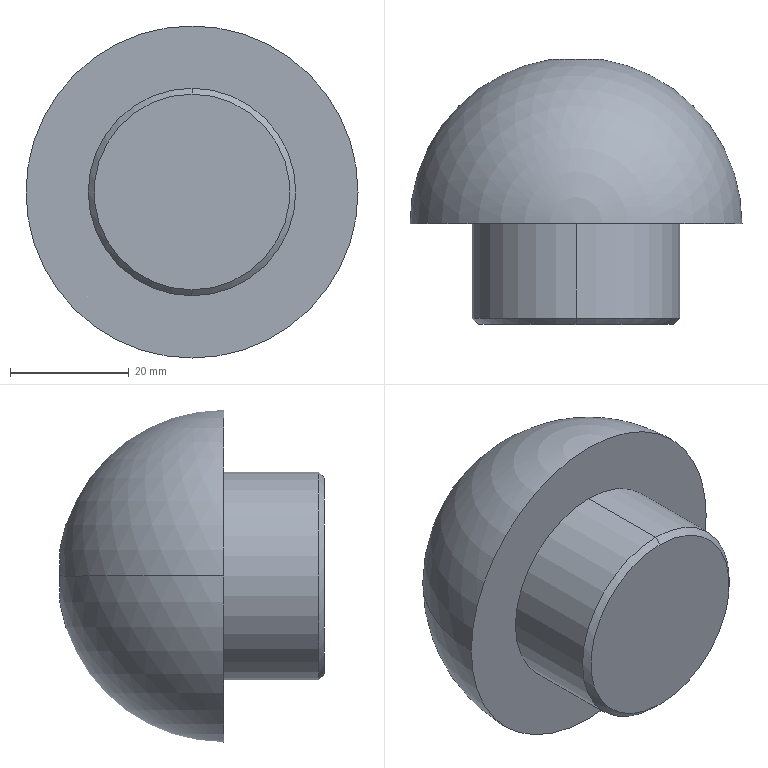Part | SolidWorks | features MirrorStock 1 | 1 solid | 12 faces | box 56 x 44.676 x 56 mm | volume 61558 mm3 | cone 4 | cylinder 4 | sphere 2 | plane 2 | commonest cylinder face diameters 8.5 x2 35 x2
STEP:
#1=CARTESIAN_POINT('',(0.,-17.,-16.5));
#2=VERTEX_POINT('',#1);
#3=CARTESIAN_POINT('',(0.,-17.,16.5));
#4=VERTEX_POINT('',#3);
#5=CARTESIAN_POINT('',(0.,-17.,0.));
#6=DIRECTION('',(0.,1.,0.));
#7=DIRECTION('',(0.,0.,1.));
#8=AXIS2_PLACEMENT_3D('',#5,#6,#7);
#9=CIRCLE('',#8,16.5);
#10=EDGE_CURVE('',#2,#4,#9,.T.);
#11=ORIENTED_EDGE('',*,*,#10,.T.);
#12=CARTESIAN_POINT('',(0.,-16.,17.5));
#13=VERTEX_POINT('',#12);
#14=CARTESIAN_POINT('',(0.,-17.,16.5));
#15=DIRECTION('',(0.,0.7071,0.7071));
#16=VECTOR('',#15,1000.);
#17=LINE('',#14,#16);
#18=EDGE_CURVE('',#4,#13,#17,.T.);
#19=ORIENTED_EDGE('',*,*,#18,.T.);
#20=CARTESIAN_POINT('',(0.,-16.,-17.5));
#21=VERTEX_POINT('',#20);
#22=CARTESIAN_POINT('',(0.,-16.,0.));
#23=DIRECTION('',(0.,-1.,0.));
#24=DIRECTION('',(0.,0.,1.));
#25=AXIS2_PLACEMENT_3D('',#22,#23,#24);
#26=CIRCLE('',#25,17.5);
#27=EDGE_CURVE('',#13,#21,#26,.T.);
#28=ORIENTED_EDGE('',*,*,#27,.T.);
#29=CARTESIAN_POINT('',(0.,-17.,-16.5));
#30=DIRECTION('',(0.,0.7071,-0.7071));
#31=VECTOR('',#30,1000.);
#32=LINE('',#29,#31);
#33=EDGE_CURVE('',#2,#21,#32,.T.);
#34=ORIENTED_EDGE('',*,*,#33,.F.);
#35=EDGE_LOOP('',(#11,#19,#28,#34));
#36=FACE_OUTER_BOUND('',#35,.T.);
#37=CARTESIAN_POINT('',(0.,-17.,0.));
#38=DIRECTION('',(0.,1.,0.));
#39=DIRECTION('',(0.,0.,-1.));
#40=AXIS2_PLACEMENT_3D('',#37,#38,#39);
#41=CONICAL_SURFACE('',#40,16.5,0.7854);
#42=ADVANCED_FACE('',(#36),#41,.T.);
#43=CARTESIAN_POINT('',(0.,16.,-4.25));
#44=VERTEX_POINT('',#43);
#45=CARTESIAN_POINT('',(0.,16.,4.25));
#46=VERTEX_POINT('',#45);
#47=CARTESIAN_POINT('',(0.,16.,0.));
#48=DIRECTION('',(0.,-1.,0.));
#49=DIRECTION('',(0.,0.,-1.));
#50=AXIS2_PLACEMENT_3D('',#47,#48,#49);
#51=CIRCLE('',#50,4.25);
#52=EDGE_CURVE('',#44,#46,#51,.T.);
#53=ORIENTED_EDGE('',*,*,#52,.T.);
#54=CARTESIAN_POINT('',(0.,27.676,4.25));
#55=VERTEX_POINT('',#54);
#56=CARTESIAN_POINT('',(0.,28.,4.25));
#57=DIRECTION('',(0.,1.,0.));
#58=VECTOR('',#57,1000.);
#59=LINE('',#56,#58);
#60=EDGE_CURVE('',#46,#55,#59,.T.);
#61=ORIENTED_EDGE('',*,*,#60,.T.);
#62=CARTESIAN_POINT('',(4.25,27.676,0.));
#63=VERTEX_POINT('',#62);
#64=CARTESIAN_POINT('',(0.,27.676,0.));
#65=DIRECTION('',(0.,-1.,0.));
#66=DIRECTION('',(0.,0.,1.));
#67=AXIS2_PLACEMENT_3D('',#64,#65,#66);
#68=CIRCLE('',#67,4.25);
#69=EDGE_CURVE('',#63,#55,#68,.T.);
#70=ORIENTED_EDGE('',*,*,#69,.F.);
#71=CARTESIAN_POINT('',(0.,27.676,-4.25));
#72=VERTEX_POINT('',#71);
#73=CARTESIAN_POINT('',(0.,27.676,0.));
#74=DIRECTION('',(0.,-1.,0.));
#75=DIRECTION('',(0.,0.,1.));
#76=AXIS2_PLACEMENT_3D('',#73,#74,#75);
#77=CIRCLE('',#76,4.25);
#78=EDGE_CURVE('',#72,#63,#77,.T.);
#79=ORIENTED_EDGE('',*,*,#78,.F.);
#80=CARTESIAN_POINT('',(0.,28.,-4.25));
#81=DIRECTION('',(0.,1.,0.));
#82=VECTOR('',#81,1000.);
#83=LINE('',#80,#82);
#84=EDGE_CURVE('',#44,#72,#83,.T.);
#85=ORIENTED_EDGE('',*,*,#84,.F.);
#86=EDGE_LOOP('',(#53,#61,#70,#79,#85));
#87=FACE_OUTER_BOUND('',#86,.T.);
#88=CARTESIAN_POINT('',(0.,28.,0.));
#89=DIRECTION('',(0.,1.,0.));
#90=DIRECTION('',(0.,0.,-1.));
#91=AXIS2_PLACEMENT_3D('',#88,#89,#90);
#92=CYLINDRICAL_SURFACE('',#91,4.25);
#93=ADVANCED_FACE('',(#87),#92,.F.);
#94=CARTESIAN_POINT('',(0.,13.446,0.));
#95=VERTEX_POINT('',#94);
#96=CARTESIAN_POINT('',(0.,16.,-4.25));
#97=DIRECTION('',(0.,0.515,-0.8572));
#98=VECTOR('',#97,1000.);
#99=LINE('',#96,#98);
#100=EDGE_CURVE('',#95,#44,#99,.T.);
#101=ORIENTED_EDGE('',*,*,#100,.F.);
#102=CARTESIAN_POINT('',(0.,16.,4.25));
#103=DIRECTION('',(0.,0.515,0.8572));
#104=VECTOR('',#103,1000.);
#105=LINE('',#102,#104);
#106=EDGE_CURVE('',#95,#46,#105,.T.);
#107=ORIENTED_EDGE('',*,*,#106,.T.);
#108=ORIENTED_EDGE('',*,*,#52,.F.);
#109=EDGE_LOOP('',(#101,#107,#108));
#110=FACE_OUTER_BOUND('',#109,.T.);
#111=CARTESIAN_POINT('',(0.,16.,0.));
#112=DIRECTION('',(0.,1.,0.));
#113=DIRECTION('',(0.,0.,-1.));
#114=AXIS2_PLACEMENT_3D('',#111,#112,#113);
#115=CONICAL_SURFACE('',#114,4.25,1.03);
#116=ADVANCED_FACE('',(#110),#115,.F.);
#117=ORIENTED_EDGE('',*,*,#69,.T.);
#118=CARTESIAN_POINT('',(-4.25,27.676,0.));
#119=VERTEX_POINT('',#118);
#120=CARTESIAN_POINT('',(0.,27.676,0.));
#121=DIRECTION('',(0.,-1.,0.));
#122=DIRECTION('',(0.,0.,1.));
#123=AXIS2_PLACEMENT_3D('',#120,#121,#122);
#124=CIRCLE('',#123,4.25);
#125=EDGE_CURVE('',#55,#119,#124,.T.);
#126=ORIENTED_EDGE('',*,*,#125,.T.);
#127=CARTESIAN_POINT('',(-28.,0.,0.));
#128=VERTEX_POINT('',#127);
#129=CARTESIAN_POINT('',(0.,0.,0.));
#130=DIRECTION('',(0.,0.,1.));
#131=DIRECTION('',(1.,0.,0.));
#132=AXIS2_PLACEMENT_3D('',#129,#130,#131);
#133=CIRCLE('',#132,28.);
#134=EDGE_CURVE('',#119,#128,#133,.T.);
#135=ORIENTED_EDGE('',*,*,#134,.T.);
#136=CARTESIAN_POINT('',(28.,0.,0.));
#137=VERTEX_POINT('',#136);
#138=CARTESIAN_POINT('',(0.,0.,0.));
#139=DIRECTION('',(0.,1.,0.));
#140=DIRECTION('',(0.,0.,1.));
#141=AXIS2_PLACEMENT_3D('',#138,#139,#140);
#142=CIRCLE('',#141,28.);
#143=EDGE_CURVE('',#128,#137,#142,.T.);
#144=ORIENTED_EDGE('',*,*,#143,.T.);
#145=CARTESIAN_POINT('',(0.,0.,0.));
#146=DIRECTION('',(0.,0.,-1.));
#147=DIRECTION('',(-1.,0.,0.));
#148=AXIS2_PLACEMENT_3D('',#145,#146,#147);
#149=CIRCLE('',#148,28.);
#150=EDGE_CURVE('',#63,#137,#149,.T.);
#151=ORIENTED_EDGE('',*,*,#150,.F.);
#152=EDGE_LOOP('',(#117,#126,#135,#144,#151));
#153=FACE_OUTER_BOUND('',#152,.T.);
#154=CARTESIAN_POINT('',(0.,0.,0.));
#155=DIRECTION('',(0.,0.,1.));
#156=DIRECTION('',(1.,0.,0.));
#157=AXIS2_PLACEMENT_3D('',#154,#155,#156);
#158=SPHERICAL_SURFACE('',#157,28.);
#159=ADVANCED_FACE('',(#153),#158,.T.);
#160=CARTESIAN_POINT('',(0.,0.,-17.5));
#161=VERTEX_POINT('',#160);
#162=CARTESIAN_POINT('',(0.,0.,17.5));
#163=VERTEX_POINT('',#162);
#164=CARTESIAN_POINT('',(0.,0.,0.));
#165=DIRECTION('',(0.,1.,0.));
#166=DIRECTION('',(0.,0.,1.));
#167=AXIS2_PLACEMENT_3D('',#164,#165,#166);
#168=CIRCLE('',#167,17.5);
#169=EDGE_CURVE('',#161,#163,#168,.T.);
#170=ORIENTED_EDGE('',*,*,#169,.F.);
#171=CARTESIAN_POINT('',(0.,0.,-17.5));
#172=DIRECTION('',(0.,-1.,0.));
#173=VECTOR('',#172,1000.);
#174=LINE('',#171,#173);
#175=EDGE_CURVE('',#161,#21,#174,.T.);
#176=ORIENTED_EDGE('',*,*,#175,.T.);
#177=ORIENTED_EDGE('',*,*,#27,.F.);
#178=CARTESIAN_POINT('',(0.,0.,17.5));
#179=DIRECTION('',(0.,-1.,0.));
#180=VECTOR('',#179,1000.);
#181=LINE('',#178,#180);
#182=EDGE_CURVE('',#163,#13,#181,.T.);
#183=ORIENTED_EDGE('',*,*,#182,.F.);
#184=EDGE_LOOP('',(#170,#176,#177,#183));
#185=FACE_OUTER_BOUND('',#184,.T.);
#186=CARTESIAN_POINT('',(0.,0.,0.));
#187=DIRECTION('',(0.,-1.,0.));
#188=DIRECTION('',(0.,0.,1.));
#189=AXIS2_PLACEMENT_3D('',#186,#187,#188);
#190=CYLINDRICAL_SURFACE('',#189,17.5);
#191=ADVANCED_FACE('',(#185),#190,.T.);
#192=ORIENTED_EDGE('',*,*,#175,.F.);
#193=CARTESIAN_POINT('',(0.,0.,0.));
#194=DIRECTION('',(0.,1.,0.));
#195=DIRECTION('',(0.,0.,1.));
#196=AXIS2_PLACEMENT_3D('',#193,#194,#195);
#197=CIRCLE('',#196,17.5);
#198=EDGE_CURVE('',#163,#161,#197,.T.);
#199=ORIENTED_EDGE('',*,*,#198,.F.);
#200=ORIENTED_EDGE('',*,*,#182,.T.);
#201=CARTESIAN_POINT('',(0.,-16.,0.));
#202=DIRECTION('',(0.,-1.,0.));
#203=DIRECTION('',(0.,0.,1.));
#204=AXIS2_PLACEMENT_3D('',#201,#202,#203);
#205=CIRCLE('',#204,17.5);
#206=EDGE_CURVE('',#21,#13,#205,.T.);
#207=ORIENTED_EDGE('',*,*,#206,.F.);
#208=EDGE_LOOP('',(#192,#199,#200,#207));
#209=FACE_OUTER_BOUND('',#208,.T.);
#210=CARTESIAN_POINT('',(0.,0.,0.));
#211=DIRECTION('',(0.,-1.,0.));
#212=DIRECTION('',(0.,0.,1.));
#213=AXIS2_PLACEMENT_3D('',#210,#211,#212);
#214=CYLINDRICAL_SURFACE('',#213,17.5);
#215=ADVANCED_FACE('',(#209),#214,.T.);
#216=CARTESIAN_POINT('',(0.,0.,0.));
#217=DIRECTION('',(0.,1.,0.));
#218=DIRECTION('',(0.,0.,1.));
#219=AXIS2_PLACEMENT_3D('',#216,#217,#218);
#220=CIRCLE('',#219,28.);
#221=EDGE_CURVE('',#137,#128,#220,.T.);
#222=ORIENTED_EDGE('',*,*,#221,.F.);
#223=ORIENTED_EDGE('',*,*,#143,.F.);
#224=EDGE_LOOP('',(#222,#223));
#225=FACE_OUTER_BOUND('',#224,.T.);
#226=ORIENTED_EDGE('',*,*,#198,.T.);
#227=ORIENTED_EDGE('',*,*,#169,.T.);
#228=EDGE_LOOP('',(#226,#227));
#229=FACE_BOUND('',#228,.T.);
#230=CARTESIAN_POINT('',(17.5,0.,0.));
#231=DIRECTION('',(0.,-1.,0.));
#232=DIRECTION('',(0.,0.,1.));
#233=AXIS2_PLACEMENT_3D('',#230,#231,#232);
#234=PLANE('',#233);
#235=ADVANCED_FACE('',(#225,#229),#234,.T.);
#236=ORIENTED_EDGE('',*,*,#134,.F.);
#237=CARTESIAN_POINT('',(0.,27.676,0.));
#238=DIRECTION('',(0.,-1.,0.));
#239=DIRECTION('',(0.,0.,1.));
#240=AXIS2_PLACEMENT_3D('',#237,#238,#239);
#241=CIRCLE('',#240,4.25);
#242=EDGE_CURVE('',#119,#72,#241,.T.);
#243=ORIENTED_EDGE('',*,*,#242,.T.);
#244=ORIENTED_EDGE('',*,*,#78,.T.);
#245=ORIENTED_EDGE('',*,*,#150,.T.);
#246=ORIENTED_EDGE('',*,*,#221,.T.);
#247=EDGE_LOOP('',(#236,#243,#244,#245,#246));
#248=FACE_OUTER_BOUND('',#247,.T.);
#249=CARTESIAN_POINT('',(0.,0.,0.));
#250=DIRECTION('',(0.,0.,1.));
#251=DIRECTION('',(1.,0.,0.));
#252=AXIS2_PLACEMENT_3D('',#249,#250,#251);
#253=SPHERICAL_SURFACE('',#252,28.);
#254=ADVANCED_FACE('',(#248),#253,.T.);
#255=ORIENTED_EDGE('',*,*,#10,.F.);
#256=CARTESIAN_POINT('',(0.,-17.,0.));
#257=DIRECTION('',(0.,1.,0.));
#258=DIRECTION('',(0.,0.,1.));
#259=AXIS2_PLACEMENT_3D('',#256,#257,#258);
#260=CIRCLE('',#259,16.5);
#261=EDGE_CURVE('',#4,#2,#260,.T.);
#262=ORIENTED_EDGE('',*,*,#261,.F.);
#263=EDGE_LOOP('',(#255,#262));
#264=FACE_OUTER_BOUND('',#263,.T.);
#265=CARTESIAN_POINT('',(0.,-17.,0.));
#266=DIRECTION('',(0.,-1.,0.));
#267=DIRECTION('',(0.,0.,1.));
#268=AXIS2_PLACEMENT_3D('',#265,#266,#267);
#269=PLANE('',#268);
#270=ADVANCED_FACE('',(#264),#269,.T.);
#271=ORIENTED_EDGE('',*,*,#106,.F.);
#272=ORIENTED_EDGE('',*,*,#100,.T.);
#273=CARTESIAN_POINT('',(0.,16.,0.));
#274=DIRECTION('',(0.,-1.,0.));
#275=DIRECTION('',(0.,0.,-1.));
#276=AXIS2_PLACEMENT_3D('',#273,#274,#275);
#277=CIRCLE('',#276,4.25);
#278=EDGE_CURVE('',#46,#44,#277,.T.);
#279=ORIENTED_EDGE('',*,*,#278,.F.);
#280=EDGE_LOOP('',(#271,#272,#279));
#281=FACE_OUTER_BOUND('',#280,.T.);
#282=CARTESIAN_POINT('',(0.,16.,0.));
#283=DIRECTION('',(0.,1.,0.));
#284=DIRECTION('',(0.,0.,-1.));
#285=AXIS2_PLACEMENT_3D('',#282,#283,#284);
#286=CONICAL_SURFACE('',#285,4.25,1.03);
#287=ADVANCED_FACE('',(#281),#286,.F.);
#288=ORIENTED_EDGE('',*,*,#60,.F.);
#289=ORIENTED_EDGE('',*,*,#278,.T.);
#290=ORIENTED_EDGE('',*,*,#84,.T.);
#291=ORIENTED_EDGE('',*,*,#242,.F.);
#292=ORIENTED_EDGE('',*,*,#125,.F.);
#293=EDGE_LOOP('',(#288,#289,#290,#291,#292));
#294=FACE_OUTER_BOUND('',#293,.T.);
#295=CARTESIAN_POINT('',(0.,28.,0.));
#296=DIRECTION('',(0.,1.,0.));
#297=DIRECTION('',(0.,0.,-1.));
#298=AXIS2_PLACEMENT_3D('',#295,#296,#297);
#299=CYLINDRICAL_SURFACE('',#298,4.25);
#300=ADVANCED_FACE('',(#294),#299,.F.);
#301=ORIENTED_EDGE('',*,*,#18,.F.);
#302=ORIENTED_EDGE('',*,*,#261,.T.);
#303=ORIENTED_EDGE('',*,*,#33,.T.);
#304=ORIENTED_EDGE('',*,*,#206,.T.);
#305=EDGE_LOOP('',(#301,#302,#303,#304));
#306=FACE_OUTER_BOUND('',#305,.T.);
#307=CARTESIAN_POINT('',(0.,-17.,0.));
#308=DIRECTION('',(0.,1.,0.));
#309=DIRECTION('',(0.,0.,-1.));
#310=AXIS2_PLACEMENT_3D('',#307,#308,#309);
#311=CONICAL_SURFACE('',#310,16.5,0.7854);
#312=ADVANCED_FACE('',(#306),#311,.T.);
#313=CLOSED_SHELL('',(#42,#93,#116,#159,#191,#215,#235,#254,#270,#287,#300,#312));
#314=MANIFOLD_SOLID_BREP('',#313);
#315=CARTESIAN_POINT('',(0.,0.,0.));
#316=DIRECTION('',(0.,0.,1.));
#317=DIRECTION('',(1.,0.,0.));
#318=AXIS2_PLACEMENT_3D('',#315,#316,#317);
#319=(LENGTH_UNIT()NAMED_UNIT(*)SI_UNIT(.MILLI.,.METRE.));
#320=UNCERTAINTY_MEASURE_WITH_UNIT(LENGTH_MEASURE(0.00001),#319,'','');
#321=(NAMED_UNIT(*)PLANE_ANGLE_UNIT()SI_UNIT($,.RADIAN.));
#322=(NAMED_UNIT(*)SI_UNIT($,.STERADIAN.)SOLID_ANGLE_UNIT());
#323=(GEOMETRIC_REPRESENTATION_CONTEXT(3)GLOBAL_UNCERTAINTY_ASSIGNED_CONTEXT((#320))GLOBAL_UNIT_ASSIGNED_CONTEXT((#319,#321,#322))REPRESENTATION_CONTEXT('',''));
#324=ADVANCED_BREP_SHAPE_REPRESENTATION('',(#314,#318),#323);